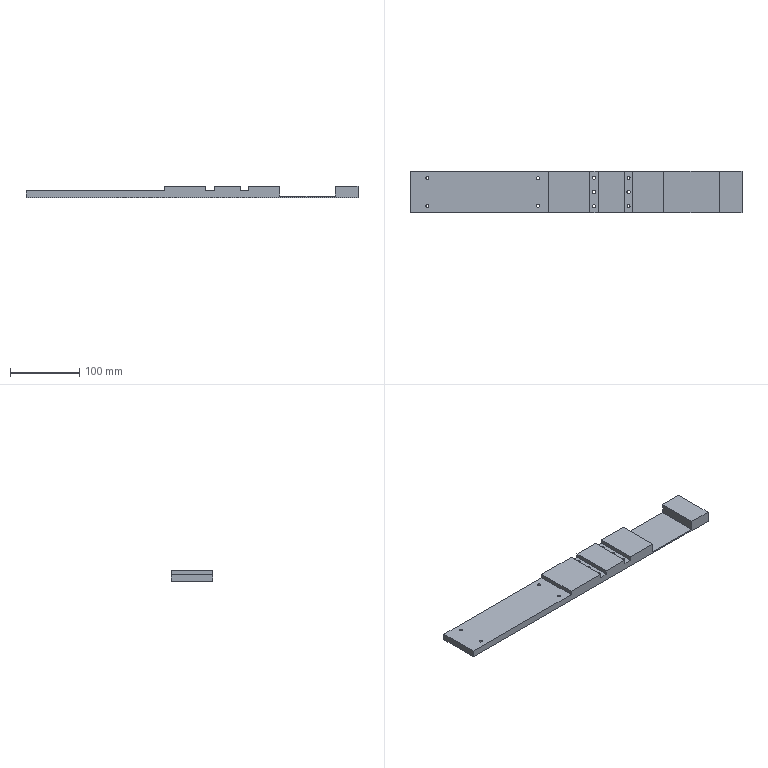Part | SolidWorks | features ICE 4, Extrusion 1 | 1 solid | 40 faces | box 480 x 60 x 16 mm | volume 311459 mm3 | cylinder 20 | plane 20 | commonest cylinder face diameters 4.2 x16 5 x4
STEP:
#1=CARTESIAN_POINT('',(-136.908,-22.163,0.));
#2=VERTEX_POINT('',#1);
#3=CARTESIAN_POINT('',(-132.708,-22.163,0.));
#4=VERTEX_POINT('',#3);
#5=CARTESIAN_POINT('',(-134.808,-22.163,0.));
#6=DIRECTION('',(0.,0.,1.));
#7=DIRECTION('',(1.,0.,0.));
#8=AXIS2_PLACEMENT_3D('',#5,#6,#7);
#9=CIRCLE('',#8,2.1);
#10=EDGE_CURVE('',#2,#4,#9,.T.);
#11=ORIENTED_EDGE('',*,*,#10,.F.);
#12=CARTESIAN_POINT('',(-136.908,-22.163,10.));
#13=VERTEX_POINT('',#12);
#14=CARTESIAN_POINT('',(-136.908,-22.163,0.));
#15=DIRECTION('',(0.,0.,1.));
#16=VECTOR('',#15,1000.);
#17=LINE('',#14,#16);
#18=EDGE_CURVE('',#2,#13,#17,.T.);
#19=ORIENTED_EDGE('',*,*,#18,.T.);
#20=CARTESIAN_POINT('',(-132.708,-22.163,10.));
#21=VERTEX_POINT('',#20);
#22=CARTESIAN_POINT('',(-134.808,-22.163,10.));
#23=DIRECTION('',(0.,0.,1.));
#24=DIRECTION('',(1.,0.,0.));
#25=AXIS2_PLACEMENT_3D('',#22,#23,#24);
#26=CIRCLE('',#25,2.1);
#27=EDGE_CURVE('',#13,#21,#26,.T.);
#28=ORIENTED_EDGE('',*,*,#27,.T.);
#29=CARTESIAN_POINT('',(-132.708,-22.163,0.));
#30=DIRECTION('',(0.,0.,1.));
#31=VECTOR('',#30,1000.);
#32=LINE('',#29,#31);
#33=EDGE_CURVE('',#4,#21,#32,.T.);
#34=ORIENTED_EDGE('',*,*,#33,.F.);
#35=EDGE_LOOP('',(#11,#19,#28,#34));
#36=FACE_OUTER_BOUND('',#35,.T.);
#37=CARTESIAN_POINT('',(-134.808,-22.163,0.));
#38=DIRECTION('',(0.,0.,1.));
#39=DIRECTION('',(1.,0.,0.));
#40=AXIS2_PLACEMENT_3D('',#37,#38,#39);
#41=CYLINDRICAL_SURFACE('',#40,2.1);
#42=ADVANCED_FACE('',(#36),#41,.F.);
#43=CARTESIAN_POINT('',(23.092,17.837,0.));
#44=VERTEX_POINT('',#43);
#45=CARTESIAN_POINT('',(27.292,17.837,0.));
#46=VERTEX_POINT('',#45);
#47=CARTESIAN_POINT('',(25.192,17.837,0.));
#48=DIRECTION('',(0.,0.,1.));
#49=DIRECTION('',(1.,0.,0.));
#50=AXIS2_PLACEMENT_3D('',#47,#48,#49);
#51=CIRCLE('',#50,2.1);
#52=EDGE_CURVE('',#44,#46,#51,.T.);
#53=ORIENTED_EDGE('',*,*,#52,.F.);
#54=CARTESIAN_POINT('',(23.092,17.837,10.));
#55=VERTEX_POINT('',#54);
#56=CARTESIAN_POINT('',(23.092,17.837,0.));
#57=DIRECTION('',(0.,0.,1.));
#58=VECTOR('',#57,1000.);
#59=LINE('',#56,#58);
#60=EDGE_CURVE('',#44,#55,#59,.T.);
#61=ORIENTED_EDGE('',*,*,#60,.T.);
#62=CARTESIAN_POINT('',(27.292,17.837,10.));
#63=VERTEX_POINT('',#62);
#64=CARTESIAN_POINT('',(25.192,17.837,10.));
#65=DIRECTION('',(0.,0.,1.));
#66=DIRECTION('',(1.,0.,0.));
#67=AXIS2_PLACEMENT_3D('',#64,#65,#66);
#68=CIRCLE('',#67,2.1);
#69=EDGE_CURVE('',#55,#63,#68,.T.);
#70=ORIENTED_EDGE('',*,*,#69,.T.);
#71=CARTESIAN_POINT('',(27.292,17.837,0.));
#72=DIRECTION('',(0.,0.,1.));
#73=VECTOR('',#72,1000.);
#74=LINE('',#71,#73);
#75=EDGE_CURVE('',#46,#63,#74,.T.);
#76=ORIENTED_EDGE('',*,*,#75,.F.);
#77=EDGE_LOOP('',(#53,#61,#70,#76));
#78=FACE_OUTER_BOUND('',#77,.T.);
#79=CARTESIAN_POINT('',(25.192,17.837,0.));
#80=DIRECTION('',(0.,0.,1.));
#81=DIRECTION('',(1.,0.,0.));
#82=AXIS2_PLACEMENT_3D('',#79,#80,#81);
#83=CYLINDRICAL_SURFACE('',#82,2.1);
#84=ADVANCED_FACE('',(#78),#83,.F.);
#85=CARTESIAN_POINT('',(23.092,-22.163,0.));
#86=VERTEX_POINT('',#85);
#87=CARTESIAN_POINT('',(27.292,-22.163,0.));
#88=VERTEX_POINT('',#87);
#89=CARTESIAN_POINT('',(25.192,-22.163,0.));
#90=DIRECTION('',(0.,0.,1.));
#91=DIRECTION('',(1.,0.,0.));
#92=AXIS2_PLACEMENT_3D('',#89,#90,#91);
#93=CIRCLE('',#92,2.1);
#94=EDGE_CURVE('',#86,#88,#93,.T.);
#95=ORIENTED_EDGE('',*,*,#94,.F.);
#96=CARTESIAN_POINT('',(23.092,-22.163,10.));
#97=VERTEX_POINT('',#96);
#98=CARTESIAN_POINT('',(23.092,-22.163,0.));
#99=DIRECTION('',(0.,0.,1.));
#100=VECTOR('',#99,1000.);
#101=LINE('',#98,#100);
#102=EDGE_CURVE('',#86,#97,#101,.T.);
#103=ORIENTED_EDGE('',*,*,#102,.T.);
#104=CARTESIAN_POINT('',(27.292,-22.163,10.));
#105=VERTEX_POINT('',#104);
#106=CARTESIAN_POINT('',(25.192,-22.163,10.));
#107=DIRECTION('',(0.,0.,1.));
#108=DIRECTION('',(1.,0.,0.));
#109=AXIS2_PLACEMENT_3D('',#106,#107,#108);
#110=CIRCLE('',#109,2.1);
#111=EDGE_CURVE('',#97,#105,#110,.T.);
#112=ORIENTED_EDGE('',*,*,#111,.T.);
#113=CARTESIAN_POINT('',(27.292,-22.163,0.));
#114=DIRECTION('',(0.,0.,1.));
#115=VECTOR('',#114,1000.);
#116=LINE('',#113,#115);
#117=EDGE_CURVE('',#88,#105,#116,.T.);
#118=ORIENTED_EDGE('',*,*,#117,.F.);
#119=EDGE_LOOP('',(#95,#103,#112,#118));
#120=FACE_OUTER_BOUND('',#119,.T.);
#121=CARTESIAN_POINT('',(25.192,-22.163,0.));
#122=DIRECTION('',(0.,0.,1.));
#123=DIRECTION('',(1.,0.,0.));
#124=AXIS2_PLACEMENT_3D('',#121,#122,#123);
#125=CYLINDRICAL_SURFACE('',#124,2.1);
#126=ADVANCED_FACE('',(#120),#125,.F.);
#127=CARTESIAN_POINT('',(-136.908,17.837,0.));
#128=VERTEX_POINT('',#127);
#129=CARTESIAN_POINT('',(-132.708,17.837,0.));
#130=VERTEX_POINT('',#129);
#131=CARTESIAN_POINT('',(-134.808,17.837,0.));
#132=DIRECTION('',(0.,0.,1.));
#133=DIRECTION('',(1.,0.,0.));
#134=AXIS2_PLACEMENT_3D('',#131,#132,#133);
#135=CIRCLE('',#134,2.1);
#136=EDGE_CURVE('',#128,#130,#135,.T.);
#137=ORIENTED_EDGE('',*,*,#136,.F.);
#138=CARTESIAN_POINT('',(-136.908,17.837,10.));
#139=VERTEX_POINT('',#138);
#140=CARTESIAN_POINT('',(-136.908,17.837,0.));
#141=DIRECTION('',(0.,0.,1.));
#142=VECTOR('',#141,1000.);
#143=LINE('',#140,#142);
#144=EDGE_CURVE('',#128,#139,#143,.T.);
#145=ORIENTED_EDGE('',*,*,#144,.T.);
#146=CARTESIAN_POINT('',(-132.708,17.837,10.));
#147=VERTEX_POINT('',#146);
#148=CARTESIAN_POINT('',(-134.808,17.837,10.));
#149=DIRECTION('',(0.,0.,1.));
#150=DIRECTION('',(1.,0.,0.));
#151=AXIS2_PLACEMENT_3D('',#148,#149,#150);
#152=CIRCLE('',#151,2.1);
#153=EDGE_CURVE('',#139,#147,#152,.T.);
#154=ORIENTED_EDGE('',*,*,#153,.T.);
#155=CARTESIAN_POINT('',(-132.708,17.837,0.));
#156=DIRECTION('',(0.,0.,1.));
#157=VECTOR('',#156,1000.);
#158=LINE('',#155,#157);
#159=EDGE_CURVE('',#130,#147,#158,.T.);
#160=ORIENTED_EDGE('',*,*,#159,.F.);
#161=EDGE_LOOP('',(#137,#145,#154,#160));
#162=FACE_OUTER_BOUND('',#161,.T.);
#163=CARTESIAN_POINT('',(-134.808,17.837,0.));
#164=DIRECTION('',(0.,0.,1.));
#165=DIRECTION('',(1.,0.,0.));
#166=AXIS2_PLACEMENT_3D('',#163,#164,#165);
#167=CYLINDRICAL_SURFACE('',#166,2.1);
#168=ADVANCED_FACE('',(#162),#167,.F.);
#169=CARTESIAN_POINT('',(154.092,18.337,0.));
#170=VERTEX_POINT('',#169);
#171=CARTESIAN_POINT('',(158.292,18.337,0.));
#172=VERTEX_POINT('',#171);
#173=CARTESIAN_POINT('',(156.192,18.337,0.));
#174=DIRECTION('',(0.,0.,1.));
#175=DIRECTION('',(1.,0.,0.));
#176=AXIS2_PLACEMENT_3D('',#173,#174,#175);
#177=CIRCLE('',#176,2.1);
#178=EDGE_CURVE('',#170,#172,#177,.T.);
#179=ORIENTED_EDGE('',*,*,#178,.F.);
#180=CARTESIAN_POINT('',(154.092,18.337,10.));
#181=VERTEX_POINT('',#180);
#182=CARTESIAN_POINT('',(154.092,18.337,0.));
#183=DIRECTION('',(0.,0.,1.));
#184=VECTOR('',#183,1000.);
#185=LINE('',#182,#184);
#186=EDGE_CURVE('',#170,#181,#185,.T.);
#187=ORIENTED_EDGE('',*,*,#186,.T.);
#188=CARTESIAN_POINT('',(158.292,18.337,10.));
#189=VERTEX_POINT('',#188);
#190=CARTESIAN_POINT('',(156.192,18.337,10.));
#191=DIRECTION('',(0.,0.,1.));
#192=DIRECTION('',(1.,0.,0.));
#193=AXIS2_PLACEMENT_3D('',#190,#191,#192);
#194=CIRCLE('',#193,2.1);
#195=EDGE_CURVE('',#181,#189,#194,.T.);
#196=ORIENTED_EDGE('',*,*,#195,.T.);
#197=CARTESIAN_POINT('',(158.292,18.337,0.));
#198=DIRECTION('',(0.,0.,1.));
#199=VECTOR('',#198,1000.);
#200=LINE('',#197,#199);
#201=EDGE_CURVE('',#172,#189,#200,.T.);
#202=ORIENTED_EDGE('',*,*,#201,.F.);
#203=EDGE_LOOP('',(#179,#187,#196,#202));
#204=FACE_OUTER_BOUND('',#203,.T.);
#205=CARTESIAN_POINT('',(156.192,18.337,0.));
#206=DIRECTION('',(0.,0.,1.));
#207=DIRECTION('',(1.,0.,0.));
#208=AXIS2_PLACEMENT_3D('',#205,#206,#207);
#209=CYLINDRICAL_SURFACE('',#208,2.1);
#210=ADVANCED_FACE('',(#204),#209,.F.);
#211=CARTESIAN_POINT('',(154.092,-22.663,0.));
#212=VERTEX_POINT('',#211);
#213=CARTESIAN_POINT('',(158.292,-22.663,0.));
#214=VERTEX_POINT('',#213);
#215=CARTESIAN_POINT('',(156.192,-22.663,0.));
#216=DIRECTION('',(0.,0.,1.));
#217=DIRECTION('',(1.,0.,0.));
#218=AXIS2_PLACEMENT_3D('',#215,#216,#217);
#219=CIRCLE('',#218,2.1);
#220=EDGE_CURVE('',#212,#214,#219,.T.);
#221=ORIENTED_EDGE('',*,*,#220,.F.);
#222=CARTESIAN_POINT('',(154.092,-22.663,10.));
#223=VERTEX_POINT('',#222);
#224=CARTESIAN_POINT('',(154.092,-22.663,0.));
#225=DIRECTION('',(0.,0.,1.));
#226=VECTOR('',#225,1000.);
#227=LINE('',#224,#226);
#228=EDGE_CURVE('',#212,#223,#227,.T.);
#229=ORIENTED_EDGE('',*,*,#228,.T.);
#230=CARTESIAN_POINT('',(158.292,-22.663,10.));
#231=VERTEX_POINT('',#230);
#232=CARTESIAN_POINT('',(156.192,-22.663,10.));
#233=DIRECTION('',(0.,0.,1.));
#234=DIRECTION('',(1.,0.,0.));
#235=AXIS2_PLACEMENT_3D('',#232,#233,#234);
#236=CIRCLE('',#235,2.1);
#237=EDGE_CURVE('',#223,#231,#236,.T.);
#238=ORIENTED_EDGE('',*,*,#237,.T.);
#239=CARTESIAN_POINT('',(158.292,-22.663,0.));
#240=DIRECTION('',(0.,0.,1.));
#241=VECTOR('',#240,1000.);
#242=LINE('',#239,#241);
#243=EDGE_CURVE('',#214,#231,#242,.T.);
#244=ORIENTED_EDGE('',*,*,#243,.F.);
#245=EDGE_LOOP('',(#221,#229,#238,#244));
#246=FACE_OUTER_BOUND('',#245,.T.);
#247=CARTESIAN_POINT('',(156.192,-22.663,0.));
#248=DIRECTION('',(0.,0.,1.));
#249=DIRECTION('',(1.,0.,0.));
#250=AXIS2_PLACEMENT_3D('',#247,#248,#249);
#251=CYLINDRICAL_SURFACE('',#250,2.1);
#252=ADVANCED_FACE('',(#246),#251,.F.);
#253=CARTESIAN_POINT('',(153.692,-2.163,0.));
#254=VERTEX_POINT('',#253);
#255=CARTESIAN_POINT('',(158.692,-2.163,0.));
#256=VERTEX_POINT('',#255);
#257=CARTESIAN_POINT('',(156.192,-2.163,0.));
#258=DIRECTION('',(0.,0.,1.));
#259=DIRECTION('',(1.,0.,0.));
#260=AXIS2_PLACEMENT_3D('',#257,#258,#259);
#261=CIRCLE('',#260,2.5);
#262=EDGE_CURVE('',#254,#256,#261,.T.);
#263=ORIENTED_EDGE('',*,*,#262,.F.);
#264=CARTESIAN_POINT('',(153.692,-2.163,10.));
#265=VERTEX_POINT('',#264);
#266=CARTESIAN_POINT('',(153.692,-2.163,0.));
#267=DIRECTION('',(0.,0.,1.));
#268=VECTOR('',#267,1000.);
#269=LINE('',#266,#268);
#270=EDGE_CURVE('',#254,#265,#269,.T.);
#271=ORIENTED_EDGE('',*,*,#270,.T.);
#272=CARTESIAN_POINT('',(158.692,-2.163,10.));
#273=VERTEX_POINT('',#272);
#274=CARTESIAN_POINT('',(156.192,-2.163,10.));
#275=DIRECTION('',(0.,0.,1.));
#276=DIRECTION('',(1.,0.,0.));
#277=AXIS2_PLACEMENT_3D('',#274,#275,#276);
#278=CIRCLE('',#277,2.5);
#279=EDGE_CURVE('',#265,#273,#278,.T.);
#280=ORIENTED_EDGE('',*,*,#279,.T.);
#281=CARTESIAN_POINT('',(158.692,-2.163,0.));
#282=DIRECTION('',(0.,0.,1.));
#283=VECTOR('',#282,1000.);
#284=LINE('',#281,#283);
#285=EDGE_CURVE('',#256,#273,#284,.T.);
#286=ORIENTED_EDGE('',*,*,#285,.F.);
#287=EDGE_LOOP('',(#263,#271,#280,#286));
#288=FACE_OUTER_BOUND('',#287,.T.);
#289=CARTESIAN_POINT('',(156.192,-2.163,0.));
#290=DIRECTION('',(0.,0.,1.));
#291=DIRECTION('',(1.,0.,0.));
#292=AXIS2_PLACEMENT_3D('',#289,#290,#291);
#293=CYLINDRICAL_SURFACE('',#292,2.5);
#294=ADVANCED_FACE('',(#288),#293,.F.);
#295=CARTESIAN_POINT('',(104.092,-22.663,0.));
#296=VERTEX_POINT('',#295);
#297=CARTESIAN_POINT('',(108.292,-22.663,0.));
#298=VERTEX_POINT('',#297);
#299=CARTESIAN_POINT('',(106.192,-22.663,0.));
#300=DIRECTION('',(0.,0.,1.));
#301=DIRECTION('',(1.,0.,0.));
#302=AXIS2_PLACEMENT_3D('',#299,#300,#301);
#303=CIRCLE('',#302,2.1);
#304=EDGE_CURVE('',#296,#298,#303,.T.);
#305=ORIENTED_EDGE('',*,*,#304,.F.);
#306=CARTESIAN_POINT('',(104.092,-22.663,10.));
#307=VERTEX_POINT('',#306);
#308=CARTESIAN_POINT('',(104.092,-22.663,0.));
#309=DIRECTION('',(0.,0.,1.));
#310=VECTOR('',#309,1000.);
#311=LINE('',#308,#310);
#312=EDGE_CURVE('',#296,#307,#311,.T.);
#313=ORIENTED_EDGE('',*,*,#312,.T.);
#314=CARTESIAN_POINT('',(108.292,-22.663,10.));
#315=VERTEX_POINT('',#314);
#316=CARTESIAN_POINT('',(106.192,-22.663,10.));
#317=DIRECTION('',(0.,0.,1.));
#318=DIRECTION('',(1.,0.,0.));
#319=AXIS2_PLACEMENT_3D('',#316,#317,#318);
#320=CIRCLE('',#319,2.1);
#321=EDGE_CURVE('',#307,#315,#320,.T.);
#322=ORIENTED_EDGE('',*,*,#321,.T.);
#323=CARTESIAN_POINT('',(108.292,-22.663,0.));
#324=DIRECTION('',(0.,0.,1.));
#325=VECTOR('',#324,1000.);
#326=LINE('',#323,#325);
#327=EDGE_CURVE('',#298,#315,#326,.T.);
#328=ORIENTED_EDGE('',*,*,#327,.F.);
#329=EDGE_LOOP('',(#305,#313,#322,#328));
#330=FACE_OUTER_BOUND('',#329,.T.);
#331=CARTESIAN_POINT('',(106.192,-22.663,0.));
#332=DIRECTION('',(0.,0.,1.));
#333=DIRECTION('',(1.,0.,0.));
#334=AXIS2_PLACEMENT_3D('',#331,#332,#333);
#335=CYLINDRICAL_SURFACE('',#334,2.1);
#336=ADVANCED_FACE('',(#330),#335,.F.);
#337=CARTESIAN_POINT('',(103.692,-2.163,0.));
#338=VERTEX_POINT('',#337);
#339=CARTESIAN_POINT('',(108.692,-2.163,0.));
#340=VERTEX_POINT('',#339);
#341=CARTESIAN_POINT('',(106.192,-2.163,0.));
#342=DIRECTION('',(0.,0.,1.));
#343=DIRECTION('',(1.,0.,0.));
#344=AXIS2_PLACEMENT_3D('',#341,#342,#343);
#345=CIRCLE('',#344,2.5);
#346=EDGE_CURVE('',#338,#340,#345,.T.);
#347=ORIENTED_EDGE('',*,*,#346,.F.);
#348=CARTESIAN_POINT('',(103.692,-2.163,10.));
#349=VERTEX_POINT('',#348);
#350=CARTESIAN_POINT('',(103.692,-2.163,0.));
#351=DIRECTION('',(0.,0.,1.));
#352=VECTOR('',#351,1000.);
#353=LINE('',#350,#352);
#354=EDGE_CURVE('',#338,#349,#353,.T.);
#355=ORIENTED_EDGE('',*,*,#354,.T.);
#356=CARTESIAN_POINT('',(108.692,-2.163,10.));
#357=VERTEX_POINT('',#356);
#358=CARTESIAN_POINT('',(106.192,-2.163,10.));
#359=DIRECTION('',(0.,0.,1.));
#360=DIRECTION('',(1.,0.,0.));
#361=AXIS2_PLACEMENT_3D('',#358,#359,#360);
#362=CIRCLE('',#361,2.5);
#363=EDGE_CURVE('',#349,#357,#362,.T.);
#364=ORIENTED_EDGE('',*,*,#363,.T.);
#365=CARTESIAN_POINT('',(108.692,-2.163,0.));
#366=DIRECTION('',(0.,0.,1.));
#367=VECTOR('',#366,1000.);
#368=LINE('',#365,#367);
#369=EDGE_CURVE('',#340,#357,#368,.T.);
#370=ORIENTED_EDGE('',*,*,#369,.F.);
#371=EDGE_LOOP('',(#347,#355,#364,#370));
#372=FACE_OUTER_BOUND('',#371,.T.);
#373=CARTESIAN_POINT('',(106.192,-2.163,0.));
#374=DIRECTION('',(0.,0.,1.));
#375=DIRECTION('',(1.,0.,0.));
#376=AXIS2_PLACEMENT_3D('',#373,#374,#375);
#377=CYLINDRICAL_SURFACE('',#376,2.5);
#378=ADVANCED_FACE('',(#372),#377,.F.);
#379=CARTESIAN_POINT('',(104.092,18.337,0.));
#380=VERTEX_POINT('',#379);
#381=CARTESIAN_POINT('',(108.292,18.337,0.));
#382=VERTEX_POINT('',#381);
#383=CARTESIAN_POINT('',(106.192,18.337,0.));
#384=DIRECTION('',(0.,0.,1.));
#385=DIRECTION('',(1.,0.,0.));
#386=AXIS2_PLACEMENT_3D('',#383,#384,#385);
#387=CIRCLE('',#386,2.1);
#388=EDGE_CURVE('',#380,#382,#387,.T.);
#389=ORIENTED_EDGE('',*,*,#388,.F.);
#390=CARTESIAN_POINT('',(104.092,18.337,10.));
#391=VERTEX_POINT('',#390);
#392=CARTESIAN_POINT('',(104.092,18.337,0.));
#393=DIRECTION('',(0.,0.,1.));
#394=VECTOR('',#393,1000.);
#395=LINE('',#392,#394);
#396=EDGE_CURVE('',#380,#391,#395,.T.);
#397=ORIENTED_EDGE('',*,*,#396,.T.);
#398=CARTESIAN_POINT('',(108.292,18.337,10.));
#399=VERTEX_POINT('',#398);
#400=CARTESIAN_POINT('',(106.192,18.337,10.));
#401=DIRECTION('',(0.,0.,1.));
#402=DIRECTION('',(1.,0.,0.));
#403=AXIS2_PLACEMENT_3D('',#400,#401,#402);
#404=CIRCLE('',#403,2.1);
#405=EDGE_CURVE('',#391,#399,#404,.T.);
#406=ORIENTED_EDGE('',*,*,#405,.T.);
#407=CARTESIAN_POINT('',(108.292,18.337,0.));
#408=DIRECTION('',(0.,0.,1.));
#409=VECTOR('',#408,1000.);
#410=LINE('',#407,#409);
#411=EDGE_CURVE('',#382,#399,#410,.T.);
#412=ORIENTED_EDGE('',*,*,#411,.F.);
#413=EDGE_LOOP('',(#389,#397,#406,#412));
#414=FACE_OUTER_BOUND('',#413,.T.);
#415=CARTESIAN_POINT('',(106.192,18.337,0.));
#416=DIRECTION('',(0.,0.,1.));
#417=DIRECTION('',(1.,0.,0.));
#418=AXIS2_PLACEMENT_3D('',#415,#416,#417);
#419=CYLINDRICAL_SURFACE('',#418,2.1);
#420=ADVANCED_FACE('',(#414),#419,.F.);
#421=CARTESIAN_POINT('',(287.192,-32.163,16.));
#422=VERTEX_POINT('',#421);
#423=CARTESIAN_POINT('',(287.192,27.837,16.));
#424=VERTEX_POINT('',#423);
#425=CARTESIAN_POINT('',(287.192,-32.163,16.));
#426=DIRECTION('',(0.,1.,0.));
#427=VECTOR('',#426,1000.);
#428=LINE('',#425,#427);
#429=EDGE_CURVE('',#422,#424,#428,.T.);
#430=ORIENTED_EDGE('',*,*,#429,.F.);
#431=CARTESIAN_POINT('',(320.192,-32.163,16.));
#432=VERTEX_POINT('',#431);
#433=CARTESIAN_POINT('',(320.192,-32.163,16.));
#434=DIRECTION('',(1.,0.,0.));
#435=VECTOR('',#434,1000.);
#436=LINE('',#433,#435);
#437=EDGE_CURVE('',#422,#432,#436,.T.);
#438=ORIENTED_EDGE('',*,*,#437,.T.);
#439=CARTESIAN_POINT('',(320.192,27.837,16.));
#440=VERTEX_POINT('',#439);
#441=CARTESIAN_POINT('',(320.192,-32.163,16.));
#442=DIRECTION('',(0.,1.,0.));
#443=VECTOR('',#442,1000.);
#444=LINE('',#441,#443);
#445=EDGE_CURVE('',#432,#440,#444,.T.);
#446=ORIENTED_EDGE('',*,*,#445,.T.);
#447=CARTESIAN_POINT('',(320.192,27.837,16.));
#448=DIRECTION('',(-1.,0.,0.));
#449=VECTOR('',#448,1000.);
#450=LINE('',#447,#449);
#451=EDGE_CURVE('',#440,#424,#450,.T.);
#452=ORIENTED_EDGE('',*,*,#451,.T.);
#453=EDGE_LOOP('',(#430,#438,#446,#452));
#454=FACE_OUTER_BOUND('',#453,.T.);
#455=CARTESIAN_POINT('',(0.,0.,16.));
#456=DIRECTION('',(0.,0.,1.));
#457=DIRECTION('',(1.,0.,0.));
#458=AXIS2_PLACEMENT_3D('',#455,#456,#457);
#459=PLANE('',#458);
#460=ADVANCED_FACE('',(#454),#459,.T.);
#461=CARTESIAN_POINT('',(100.192,27.837,16.));
#462=VERTEX_POINT('',#461);
#463=CARTESIAN_POINT('',(100.192,-32.163,16.));
#464=VERTEX_POINT('',#463);
#465=CARTESIAN_POINT('',(100.192,-32.163,16.));
#466=DIRECTION('',(0.,-1.,0.));
#467=VECTOR('',#466,1000.);
#468=LINE('',#465,#467);
#469=EDGE_CURVE('',#462,#464,#468,.T.);
#470=ORIENTED_EDGE('',*,*,#469,.F.);
#471=CARTESIAN_POINT('',(40.192,27.837,16.));
#472=VERTEX_POINT('',#471);
#473=CARTESIAN_POINT('',(320.192,27.837,16.));
#474=DIRECTION('',(-1.,0.,0.));
#475=VECTOR('',#474,1000.);
#476=LINE('',#473,#475);
#477=EDGE_CURVE('',#462,#472,#476,.T.);
#478=ORIENTED_EDGE('',*,*,#477,.T.);
#479=CARTESIAN_POINT('',(40.192,-32.163,16.));
#480=VERTEX_POINT('',#479);
#481=CARTESIAN_POINT('',(40.192,27.837,16.));
#482=DIRECTION('',(0.,1.,0.));
#483=VECTOR('',#482,1000.);
#484=LINE('',#481,#483);
#485=EDGE_CURVE('',#480,#472,#484,.T.);
#486=ORIENTED_EDGE('',*,*,#485,.F.);
#487=CARTESIAN_POINT('',(320.192,-32.163,16.));
#488=DIRECTION('',(1.,0.,0.));
#489=VECTOR('',#488,1000.);
#490=LINE('',#487,#489);
#491=EDGE_CURVE('',#480,#464,#490,.T.);
#492=ORIENTED_EDGE('',*,*,#491,.T.);
#493=EDGE_LOOP('',(#470,#478,#486,#492));
#494=FACE_OUTER_BOUND('',#493,.T.);
#495=CARTESIAN_POINT('',(0.,0.,16.));
#496=DIRECTION('',(0.,0.,1.));
#497=DIRECTION('',(1.,0.,0.));
#498=AXIS2_PLACEMENT_3D('',#495,#496,#497);
#499=PLANE('',#498);
#500=ADVANCED_FACE('',(#494),#499,.T.);
#501=CARTESIAN_POINT('',(112.192,-32.163,16.));
#502=VERTEX_POINT('',#501);
#503=CARTESIAN_POINT('',(112.192,27.837,16.));
#504=VERTEX_POINT('',#503);
#505=CARTESIAN_POINT('',(112.192,27.837,16.));
#506=DIRECTION('',(0.,1.,0.));
#507=VECTOR('',#506,1000.);
#508=LINE('',#505,#507);
#509=EDGE_CURVE('',#502,#504,#508,.T.);
#510=ORIENTED_EDGE('',*,*,#509,.F.);
#511=CARTESIAN_POINT('',(150.192,-32.163,16.));
#512=VERTEX_POINT('',#511);
#513=CARTESIAN_POINT('',(320.192,-32.163,16.));
#514=DIRECTION('',(1.,0.,0.));
#515=VECTOR('',#514,1000.);
#516=LINE('',#513,#515);
#517=EDGE_CURVE('',#502,#512,#516,.T.);
#518=ORIENTED_EDGE('',*,*,#517,.T.);
#519=CARTESIAN_POINT('',(150.192,27.837,16.));
#520=VERTEX_POINT('',#519);
#521=CARTESIAN_POINT('',(150.192,27.837,16.));
#522=DIRECTION('',(0.,-1.,0.));
#523=VECTOR('',#522,1000.);
#524=LINE('',#521,#523);
#525=EDGE_CURVE('',#520,#512,#524,.T.);
#526=ORIENTED_EDGE('',*,*,#525,.F.);
#527=CARTESIAN_POINT('',(320.192,27.837,16.));
#528=DIRECTION('',(-1.,0.,0.));
#529=VECTOR('',#528,1000.);
#530=LINE('',#527,#529);
#531=EDGE_CURVE('',#520,#504,#530,.T.);
#532=ORIENTED_EDGE('',*,*,#531,.T.);
#533=EDGE_LOOP('',(#510,#518,#526,#532));
#534=FACE_OUTER_BOUND('',#533,.T.);
#535=CARTESIAN_POINT('',(0.,0.,16.));
#536=DIRECTION('',(0.,0.,1.));
#537=DIRECTION('',(1.,0.,0.));
#538=AXIS2_PLACEMENT_3D('',#535,#536,#537);
#539=PLANE('',#538);
#540=ADVANCED_FACE('',(#534),#539,.T.);
#541=CARTESIAN_POINT('',(-159.808,27.837,10.));
#542=VERTEX_POINT('',#541);
#543=CARTESIAN_POINT('',(-159.808,-32.163,10.));
#544=VERTEX_POINT('',#543);
#545=CARTESIAN_POINT('',(-159.808,27.837,10.));
#546=DIRECTION('',(0.,-1.,0.));
#547=VECTOR('',#546,1000.);
#548=LINE('',#545,#547);
#549=EDGE_CURVE('',#542,#544,#548,.T.);
#550=ORIENTED_EDGE('',*,*,#549,.F.);
#551=CARTESIAN_POINT('',(-159.808,27.837,0.));
#552=VERTEX_POINT('',#551);
#553=CARTESIAN_POINT('',(-159.808,27.837,16.));
#554=DIRECTION('',(0.,0.,-1.));
#555=VECTOR('',#554,1000.);
#556=LINE('',#553,#555);
#557=EDGE_CURVE('',#542,#552,#556,.T.);
#558=ORIENTED_EDGE('',*,*,#557,.T.);
#559=CARTESIAN_POINT('',(-159.808,-32.163,0.));
#560=VERTEX_POINT('',#559);
#561=CARTESIAN_POINT('',(-159.808,-32.163,0.));
#562=DIRECTION('',(0.,-1.,0.));
#563=VECTOR('',#562,1000.);
#564=LINE('',#561,#563);
#565=EDGE_CURVE('',#552,#560,#564,.T.);
#566=ORIENTED_EDGE('',*,*,#565,.T.);
#567=CARTESIAN_POINT('',(-159.808,-32.163,16.));
#568=DIRECTION('',(0.,0.,-1.));
#569=VECTOR('',#568,1000.);
#570=LINE('',#567,#569);
#571=EDGE_CURVE('',#544,#560,#570,.T.);
#572=ORIENTED_EDGE('',*,*,#571,.F.);
#573=EDGE_LOOP('',(#550,#558,#566,#572));
#574=FACE_OUTER_BOUND('',#573,.T.);
#575=CARTESIAN_POINT('',(-159.808,-32.163,16.));
#576=DIRECTION('',(1.,0.,0.));
#577=DIRECTION('',(0.,0.,-1.));
#578=AXIS2_PLACEMENT_3D('',#575,#576,#577);
#579=PLANE('',#578);
#580=ADVANCED_FACE('',(#574),#579,.F.);
#581=CARTESIAN_POINT('',(320.192,-32.163,0.));
#582=VERTEX_POINT('',#581);
#583=CARTESIAN_POINT('',(320.192,27.837,0.));
#584=VERTEX_POINT('',#583);
#585=CARTESIAN_POINT('',(320.192,-32.163,0.));
#586=DIRECTION('',(0.,1.,0.));
#587=VECTOR('',#586,1000.);
#588=LINE('',#585,#587);
#589=EDGE_CURVE('',#582,#584,#588,.T.);
#590=ORIENTED_EDGE('',*,*,#589,.T.);
#591=CARTESIAN_POINT('',(320.192,27.837,16.));
#592=DIRECTION('',(0.,0.,-1.));
#593=VECTOR('',#592,1000.);
#594=LINE('',#591,#593);
#595=EDGE_CURVE('',#440,#584,#594,.T.);
#596=ORIENTED_EDGE('',*,*,#595,.F.);
#597=ORIENTED_EDGE('',*,*,#445,.F.);
#598=CARTESIAN_POINT('',(320.192,-32.163,16.));
#599=DIRECTION('',(0.,0.,-1.));
#600=VECTOR('',#599,1000.);
#601=LINE('',#598,#600);
#602=EDGE_CURVE('',#432,#582,#601,.T.);
#603=ORIENTED_EDGE('',*,*,#602,.T.);
#604=EDGE_LOOP('',(#590,#596,#597,#603));
#605=FACE_OUTER_BOUND('',#604,.T.);
#606=CARTESIAN_POINT('',(320.192,-32.163,16.));
#607=DIRECTION('',(-1.,0.,0.));
#608=DIRECTION('',(0.,0.,1.));
#609=AXIS2_PLACEMENT_3D('',#606,#607,#608);
#610=PLANE('',#609);
#611=ADVANCED_FACE('',(#605),#610,.F.);
#612=CARTESIAN_POINT('',(287.192,27.837,2.));
#613=VERTEX_POINT('',#612);
#614=CARTESIAN_POINT('',(207.192,27.837,2.));
#615=VERTEX_POINT('',#614);
#616=CARTESIAN_POINT('',(287.192,27.837,2.));
#617=DIRECTION('',(-1.,0.,0.));
#618=VECTOR('',#617,1000.);
#619=LINE('',#616,#618);
#620=EDGE_CURVE('',#613,#615,#619,.T.);
#621=ORIENTED_EDGE('',*,*,#620,.F.);
#622=CARTESIAN_POINT('',(287.192,27.837,2.));
#623=DIRECTION('',(0.,0.,1.));
#624=VECTOR('',#623,1000.);
#625=LINE('',#622,#624);
#626=EDGE_CURVE('',#613,#424,#625,.T.);
#627=ORIENTED_EDGE('',*,*,#626,.T.);
#628=ORIENTED_EDGE('',*,*,#451,.F.);
#629=ORIENTED_EDGE('',*,*,#595,.T.);
#630=CARTESIAN_POINT('',(320.192,27.837,0.));
#631=DIRECTION('',(-1.,0.,0.));
#632=VECTOR('',#631,1000.);
#633=LINE('',#630,#632);
#634=EDGE_CURVE('',#584,#552,#633,.T.);
#635=ORIENTED_EDGE('',*,*,#634,.T.);
#636=ORIENTED_EDGE('',*,*,#557,.F.);
#637=CARTESIAN_POINT('',(40.192,27.837,10.));
#638=VERTEX_POINT('',#637);
#639=CARTESIAN_POINT('',(-159.808,27.837,10.));
#640=DIRECTION('',(-1.,0.,0.));
#641=VECTOR('',#640,1000.);
#642=LINE('',#639,#641);
#643=EDGE_CURVE('',#638,#542,#642,.T.);
#644=ORIENTED_EDGE('',*,*,#643,.F.);
#645=CARTESIAN_POINT('',(40.192,27.837,10.));
#646=DIRECTION('',(0.,0.,1.));
#647=VECTOR('',#646,1000.);
#648=LINE('',#645,#647);
#649=EDGE_CURVE('',#638,#472,#648,.T.);
#650=ORIENTED_EDGE('',*,*,#649,.T.);
#651=ORIENTED_EDGE('',*,*,#477,.F.);
#652=CARTESIAN_POINT('',(100.192,27.837,10.));
#653=VERTEX_POINT('',#652);
#654=CARTESIAN_POINT('',(100.192,27.837,10.));
#655=DIRECTION('',(0.,0.,1.));
#656=VECTOR('',#655,1000.);
#657=LINE('',#654,#656);
#658=EDGE_CURVE('',#653,#462,#657,.T.);
#659=ORIENTED_EDGE('',*,*,#658,.F.);
#660=CARTESIAN_POINT('',(112.192,27.837,10.));
#661=VERTEX_POINT('',#660);
#662=CARTESIAN_POINT('',(100.192,27.837,10.));
#663=DIRECTION('',(-1.,0.,0.));
#664=VECTOR('',#663,1000.);
#665=LINE('',#662,#664);
#666=EDGE_CURVE('',#661,#653,#665,.T.);
#667=ORIENTED_EDGE('',*,*,#666,.F.);
#668=CARTESIAN_POINT('',(112.192,27.837,10.));
#669=DIRECTION('',(0.,0.,1.));
#670=VECTOR('',#669,1000.);
#671=LINE('',#668,#670);
#672=EDGE_CURVE('',#661,#504,#671,.T.);
#673=ORIENTED_EDGE('',*,*,#672,.T.);
#674=ORIENTED_EDGE('',*,*,#531,.F.);
#675=CARTESIAN_POINT('',(150.192,27.837,10.));
#676=VERTEX_POINT('',#675);
#677=CARTESIAN_POINT('',(150.192,27.837,10.));
#678=DIRECTION('',(0.,0.,1.));
#679=VECTOR('',#678,1000.);
#680=LINE('',#677,#679);
#681=EDGE_CURVE('',#676,#520,#680,.T.);
#682=ORIENTED_EDGE('',*,*,#681,.F.);
#683=CARTESIAN_POINT('',(162.192,27.837,10.));
#684=VERTEX_POINT('',#683);
#685=CARTESIAN_POINT('',(150.192,27.837,10.));
#686=DIRECTION('',(-1.,0.,0.));
#687=VECTOR('',#686,1000.);
#688=LINE('',#685,#687);
#689=EDGE_CURVE('',#684,#676,#688,.T.);
#690=ORIENTED_EDGE('',*,*,#689,.F.);
#691=CARTESIAN_POINT('',(162.192,27.837,16.));
#692=VERTEX_POINT('',#691);
#693=CARTESIAN_POINT('',(162.192,27.837,10.));
#694=DIRECTION('',(0.,0.,1.));
#695=VECTOR('',#694,1000.);
#696=LINE('',#693,#695);
#697=EDGE_CURVE('',#684,#692,#696,.T.);
#698=ORIENTED_EDGE('',*,*,#697,.T.);
#699=CARTESIAN_POINT('',(207.192,27.837,16.));
#700=VERTEX_POINT('',#699);
#701=CARTESIAN_POINT('',(320.192,27.837,16.));
#702=DIRECTION('',(-1.,0.,0.));
#703=VECTOR('',#702,1000.);
#704=LINE('',#701,#703);
#705=EDGE_CURVE('',#700,#692,#704,.T.);
#706=ORIENTED_EDGE('',*,*,#705,.F.);
#707=CARTESIAN_POINT('',(207.192,27.837,2.));
#708=DIRECTION('',(0.,0.,1.));
#709=VECTOR('',#708,1000.);
#710=LINE('',#707,#709);
#711=EDGE_CURVE('',#615,#700,#710,.T.);
#712=ORIENTED_EDGE('',*,*,#711,.F.);
#713=EDGE_LOOP('',(#621,#627,#628,#629,#635,#636,#644,#650,#651,#659,#667,#673,#674,#682,#690,#698,#706,#712));
#714=FACE_OUTER_BOUND('',#713,.T.);
#715=CARTESIAN_POINT('',(320.192,27.837,16.));
#716=DIRECTION('',(0.,-1.,0.));
#717=DIRECTION('',(1.,0.,0.));
#718=AXIS2_PLACEMENT_3D('',#715,#716,#717);
#719=PLANE('',#718);
#720=ADVANCED_FACE('',(#714),#719,.F.);
#721=ORIENTED_EDGE('',*,*,#437,.F.);
#722=CARTESIAN_POINT('',(287.192,-32.163,2.));
#723=VERTEX_POINT('',#722);
#724=CARTESIAN_POINT('',(287.192,-32.163,2.));
#725=DIRECTION('',(0.,0.,1.));
#726=VECTOR('',#725,1000.);
#727=LINE('',#724,#726);
#728=EDGE_CURVE('',#723,#422,#727,.T.);
#729=ORIENTED_EDGE('',*,*,#728,.F.);
#730=CARTESIAN_POINT('',(207.192,-32.163,2.));
#731=VERTEX_POINT('',#730);
#732=CARTESIAN_POINT('',(207.192,-32.163,2.));
#733=DIRECTION('',(1.,0.,0.));
#734=VECTOR('',#733,1000.);
#735=LINE('',#732,#734);
#736=EDGE_CURVE('',#731,#723,#735,.T.);
#737=ORIENTED_EDGE('',*,*,#736,.F.);
#738=CARTESIAN_POINT('',(207.192,-32.163,16.));
#739=VERTEX_POINT('',#738);
#740=CARTESIAN_POINT('',(207.192,-32.163,2.));
#741=DIRECTION('',(0.,0.,1.));
#742=VECTOR('',#741,1000.);
#743=LINE('',#740,#742);
#744=EDGE_CURVE('',#731,#739,#743,.T.);
#745=ORIENTED_EDGE('',*,*,#744,.T.);
#746=CARTESIAN_POINT('',(162.192,-32.163,16.));
#747=VERTEX_POINT('',#746);
#748=CARTESIAN_POINT('',(320.192,-32.163,16.));
#749=DIRECTION('',(1.,0.,0.));
#750=VECTOR('',#749,1000.);
#751=LINE('',#748,#750);
#752=EDGE_CURVE('',#747,#739,#751,.T.);
#753=ORIENTED_EDGE('',*,*,#752,.F.);
#754=CARTESIAN_POINT('',(162.192,-32.163,10.));
#755=VERTEX_POINT('',#754);
#756=CARTESIAN_POINT('',(162.192,-32.163,10.));
#757=DIRECTION('',(0.,0.,1.));
#758=VECTOR('',#757,1000.);
#759=LINE('',#756,#758);
#760=EDGE_CURVE('',#755,#747,#759,.T.);
#761=ORIENTED_EDGE('',*,*,#760,.F.);
#762=CARTESIAN_POINT('',(150.192,-32.163,10.));
#763=VERTEX_POINT('',#762);
#764=CARTESIAN_POINT('',(150.192,-32.163,10.));
#765=DIRECTION('',(1.,0.,0.));
#766=VECTOR('',#765,1000.);
#767=LINE('',#764,#766);
#768=EDGE_CURVE('',#763,#755,#767,.T.);
#769=ORIENTED_EDGE('',*,*,#768,.F.);
#770=CARTESIAN_POINT('',(150.192,-32.163,10.));
#771=DIRECTION('',(0.,0.,1.));
#772=VECTOR('',#771,1000.);
#773=LINE('',#770,#772);
#774=EDGE_CURVE('',#763,#512,#773,.T.);
#775=ORIENTED_EDGE('',*,*,#774,.T.);
#776=ORIENTED_EDGE('',*,*,#517,.F.);
#777=CARTESIAN_POINT('',(112.192,-32.163,10.));
#778=VERTEX_POINT('',#777);
#779=CARTESIAN_POINT('',(112.192,-32.163,10.));
#780=DIRECTION('',(0.,0.,1.));
#781=VECTOR('',#780,1000.);
#782=LINE('',#779,#781);
#783=EDGE_CURVE('',#778,#502,#782,.T.);
#784=ORIENTED_EDGE('',*,*,#783,.F.);
#785=CARTESIAN_POINT('',(100.192,-32.163,10.));
#786=VERTEX_POINT('',#785);
#787=CARTESIAN_POINT('',(112.192,-32.163,10.));
#788=DIRECTION('',(1.,0.,0.));
#789=VECTOR('',#788,1000.);
#790=LINE('',#787,#789);
#791=EDGE_CURVE('',#786,#778,#790,.T.);
#792=ORIENTED_EDGE('',*,*,#791,.F.);
#793=CARTESIAN_POINT('',(100.192,-32.163,10.));
#794=DIRECTION('',(0.,0.,1.));
#795=VECTOR('',#794,1000.);
#796=LINE('',#793,#795);
#797=EDGE_CURVE('',#786,#464,#796,.T.);
#798=ORIENTED_EDGE('',*,*,#797,.T.);
#799=ORIENTED_EDGE('',*,*,#491,.F.);
#800=CARTESIAN_POINT('',(40.192,-32.163,10.));
#801=VERTEX_POINT('',#800);
#802=CARTESIAN_POINT('',(40.192,-32.163,10.));
#803=DIRECTION('',(0.,0.,1.));
#804=VECTOR('',#803,1000.);
#805=LINE('',#802,#804);
#806=EDGE_CURVE('',#801,#480,#805,.T.);
#807=ORIENTED_EDGE('',*,*,#806,.F.);
#808=CARTESIAN_POINT('',(-159.808,-32.163,10.));
#809=DIRECTION('',(1.,0.,0.));
#810=VECTOR('',#809,1000.);
#811=LINE('',#808,#810);
#812=EDGE_CURVE('',#544,#801,#811,.T.);
#813=ORIENTED_EDGE('',*,*,#812,.F.);
#814=ORIENTED_EDGE('',*,*,#571,.T.);
#815=CARTESIAN_POINT('',(320.192,-32.163,0.));
#816=DIRECTION('',(1.,0.,0.));
#817=VECTOR('',#816,1000.);
#818=LINE('',#815,#817);
#819=EDGE_CURVE('',#560,#582,#818,.T.);
#820=ORIENTED_EDGE('',*,*,#819,.T.);
#821=ORIENTED_EDGE('',*,*,#602,.F.);
#822=EDGE_LOOP('',(#721,#729,#737,#745,#753,#761,#769,#775,#776,#784,#792,#798,#799,#807,#813,#814,#820,#821));
#823=FACE_OUTER_BOUND('',#822,.T.);
#824=CARTESIAN_POINT('',(320.192,-32.163,16.));
#825=DIRECTION('',(0.,1.,0.));
#826=DIRECTION('',(-1.,0.,0.));
#827=AXIS2_PLACEMENT_3D('',#824,#825,#826);
#828=PLANE('',#827);
#829=ADVANCED_FACE('',(#823),#828,.F.);
#830=CARTESIAN_POINT('',(207.192,27.837,16.));
#831=DIRECTION('',(0.,-1.,0.));
#832=VECTOR('',#831,1000.);
#833=LINE('',#830,#832);
#834=EDGE_CURVE('',#700,#739,#833,.T.);
#835=ORIENTED_EDGE('',*,*,#834,.F.);
#836=ORIENTED_EDGE('',*,*,#705,.T.);
#837=CARTESIAN_POINT('',(162.192,27.837,16.));
#838=DIRECTION('',(0.,1.,0.));
#839=VECTOR('',#838,1000.);
#840=LINE('',#837,#839);
#841=EDGE_CURVE('',#747,#692,#840,.T.);
#842=ORIENTED_EDGE('',*,*,#841,.F.);
#843=ORIENTED_EDGE('',*,*,#752,.T.);
#844=EDGE_LOOP('',(#835,#836,#842,#843));
#845=FACE_OUTER_BOUND('',#844,.T.);
#846=CARTESIAN_POINT('',(0.,0.,16.));
#847=DIRECTION('',(0.,0.,1.));
#848=DIRECTION('',(1.,0.,0.));
#849=AXIS2_PLACEMENT_3D('',#846,#847,#848);
#850=PLANE('',#849);
#851=ADVANCED_FACE('',(#845),#850,.T.);
#852=CARTESIAN_POINT('',(106.192,-22.663,0.));
#853=DIRECTION('',(0.,0.,1.));
#854=DIRECTION('',(1.,0.,0.));
#855=AXIS2_PLACEMENT_3D('',#852,#853,#854);
#856=CIRCLE('',#855,2.1);
#857=EDGE_CURVE('',#298,#296,#856,.T.);
#858=ORIENTED_EDGE('',*,*,#857,.T.);
#859=ORIENTED_EDGE('',*,*,#304,.T.);
#860=EDGE_LOOP('',(#858,#859));
#861=FACE_BOUND('',#860,.T.);
#862=CARTESIAN_POINT('',(156.192,18.337,0.));
#863=DIRECTION('',(0.,0.,1.));
#864=DIRECTION('',(1.,0.,0.));
#865=AXIS2_PLACEMENT_3D('',#862,#863,#864);
#866=CIRCLE('',#865,2.1);
#867=EDGE_CURVE('',#172,#170,#866,.T.);
#868=ORIENTED_EDGE('',*,*,#867,.T.);
#869=ORIENTED_EDGE('',*,*,#178,.T.);
#870=EDGE_LOOP('',(#868,#869));
#871=FACE_BOUND('',#870,.T.);
#872=CARTESIAN_POINT('',(156.192,-22.663,0.));
#873=DIRECTION('',(0.,0.,1.));
#874=DIRECTION('',(1.,0.,0.));
#875=AXIS2_PLACEMENT_3D('',#872,#873,#874);
#876=CIRCLE('',#875,2.1);
#877=EDGE_CURVE('',#214,#212,#876,.T.);
#878=ORIENTED_EDGE('',*,*,#877,.T.);
#879=ORIENTED_EDGE('',*,*,#220,.T.);
#880=EDGE_LOOP('',(#878,#879));
#881=FACE_BOUND('',#880,.T.);
#882=CARTESIAN_POINT('',(106.192,-2.163,0.));
#883=DIRECTION('',(0.,0.,1.));
#884=DIRECTION('',(1.,0.,0.));
#885=AXIS2_PLACEMENT_3D('',#882,#883,#884);
#886=CIRCLE('',#885,2.5);
#887=EDGE_CURVE('',#340,#338,#886,.T.);
#888=ORIENTED_EDGE('',*,*,#887,.T.);
#889=ORIENTED_EDGE('',*,*,#346,.T.);
#890=EDGE_LOOP('',(#888,#889));
#891=FACE_BOUND('',#890,.T.);
#892=CARTESIAN_POINT('',(-134.808,-22.163,0.));
#893=DIRECTION('',(0.,0.,1.));
#894=DIRECTION('',(1.,0.,0.));
#895=AXIS2_PLACEMENT_3D('',#892,#893,#894);
#896=CIRCLE('',#895,2.1);
#897=EDGE_CURVE('',#4,#2,#896,.T.);
#898=ORIENTED_EDGE('',*,*,#897,.T.);
#899=ORIENTED_EDGE('',*,*,#10,.T.);
#900=EDGE_LOOP('',(#898,#899));
#901=FACE_BOUND('',#900,.T.);
#902=CARTESIAN_POINT('',(25.192,17.837,0.));
#903=DIRECTION('',(0.,0.,1.));
#904=DIRECTION('',(1.,0.,0.));
#905=AXIS2_PLACEMENT_3D('',#902,#903,#904);
#906=CIRCLE('',#905,2.1);
#907=EDGE_CURVE('',#46,#44,#906,.T.);
#908=ORIENTED_EDGE('',*,*,#907,.T.);
#909=ORIENTED_EDGE('',*,*,#52,.T.);
#910=EDGE_LOOP('',(#908,#909));
#911=FACE_BOUND('',#910,.T.);
#912=CARTESIAN_POINT('',(25.192,-22.163,0.));
#913=DIRECTION('',(0.,0.,1.));
#914=DIRECTION('',(1.,0.,0.));
#915=AXIS2_PLACEMENT_3D('',#912,#913,#914);
#916=CIRCLE('',#915,2.1);
#917=EDGE_CURVE('',#88,#86,#916,.T.);
#918=ORIENTED_EDGE('',*,*,#917,.T.);
#919=ORIENTED_EDGE('',*,*,#94,.T.);
#920=EDGE_LOOP('',(#918,#919));
#921=FACE_BOUND('',#920,.T.);
#922=CARTESIAN_POINT('',(106.192,18.337,0.));
#923=DIRECTION('',(0.,0.,1.));
#924=DIRECTION('',(1.,0.,0.));
#925=AXIS2_PLACEMENT_3D('',#922,#923,#924);
#926=CIRCLE('',#925,2.1);
#927=EDGE_CURVE('',#382,#380,#926,.T.);
#928=ORIENTED_EDGE('',*,*,#927,.T.);
#929=ORIENTED_EDGE('',*,*,#388,.T.);
#930=EDGE_LOOP('',(#928,#929));
#931=FACE_BOUND('',#930,.T.);
#932=CARTESIAN_POINT('',(156.192,-2.163,0.));
#933=DIRECTION('',(0.,0.,1.));
#934=DIRECTION('',(1.,0.,0.));
#935=AXIS2_PLACEMENT_3D('',#932,#933,#934);
#936=CIRCLE('',#935,2.5);
#937=EDGE_CURVE('',#256,#254,#936,.T.);
#938=ORIENTED_EDGE('',*,*,#937,.T.);
#939=ORIENTED_EDGE('',*,*,#262,.T.);
#940=EDGE_LOOP('',(#938,#939));
#941=FACE_BOUND('',#940,.T.);
#942=CARTESIAN_POINT('',(-134.808,17.837,0.));
#943=DIRECTION('',(0.,0.,1.));
#944=DIRECTION('',(1.,0.,0.));
#945=AXIS2_PLACEMENT_3D('',#942,#943,#944);
#946=CIRCLE('',#945,2.1);
#947=EDGE_CURVE('',#130,#128,#946,.T.);
#948=ORIENTED_EDGE('',*,*,#947,.T.);
#949=ORIENTED_EDGE('',*,*,#136,.T.);
#950=EDGE_LOOP('',(#948,#949));
#951=FACE_BOUND('',#950,.T.);
#952=ORIENTED_EDGE('',*,*,#589,.F.);
#953=ORIENTED_EDGE('',*,*,#819,.F.);
#954=ORIENTED_EDGE('',*,*,#565,.F.);
#955=ORIENTED_EDGE('',*,*,#634,.F.);
#956=EDGE_LOOP('',(#952,#953,#954,#955));
#957=FACE_OUTER_BOUND('',#956,.T.);
#958=CARTESIAN_POINT('',(0.,0.,0.));
#959=DIRECTION('',(0.,0.,1.));
#960=DIRECTION('',(1.,0.,0.));
#961=AXIS2_PLACEMENT_3D('',#958,#959,#960);
#962=PLANE('',#961);
#963=ADVANCED_FACE('',(#861,#871,#881,#891,#901,#911,#921,#931,#941,#951,#957),#962,.F.);
#964=ORIENTED_EDGE('',*,*,#485,.T.);
#965=ORIENTED_EDGE('',*,*,#649,.F.);
#966=CARTESIAN_POINT('',(40.192,27.837,10.));
#967=DIRECTION('',(0.,1.,0.));
#968=VECTOR('',#967,1000.);
#969=LINE('',#966,#968);
#970=EDGE_CURVE('',#801,#638,#969,.T.);
#971=ORIENTED_EDGE('',*,*,#970,.F.);
#972=ORIENTED_EDGE('',*,*,#806,.T.);
#973=EDGE_LOOP('',(#964,#965,#971,#972));
#974=FACE_OUTER_BOUND('',#973,.T.);
#975=CARTESIAN_POINT('',(40.192,27.837,10.));
#976=DIRECTION('',(1.,0.,0.));
#977=DIRECTION('',(0.,0.,-1.));
#978=AXIS2_PLACEMENT_3D('',#975,#976,#977);
#979=PLANE('',#978);
#980=ADVANCED_FACE('',(#974),#979,.F.);
#981=CARTESIAN_POINT('',(-134.808,-22.163,10.));
#982=DIRECTION('',(0.,0.,1.));
#983=DIRECTION('',(1.,0.,0.));
#984=AXIS2_PLACEMENT_3D('',#981,#982,#983);
#985=CIRCLE('',#984,2.1);
#986=EDGE_CURVE('',#21,#13,#985,.T.);
#987=ORIENTED_EDGE('',*,*,#986,.F.);
#988=ORIENTED_EDGE('',*,*,#27,.F.);
#989=EDGE_LOOP('',(#987,#988));
#990=FACE_BOUND('',#989,.T.);
#991=CARTESIAN_POINT('',(25.192,17.837,10.));
#992=DIRECTION('',(0.,0.,1.));
#993=DIRECTION('',(1.,0.,0.));
#994=AXIS2_PLACEMENT_3D('',#991,#992,#993);
#995=CIRCLE('',#994,2.1);
#996=EDGE_CURVE('',#63,#55,#995,.T.);
#997=ORIENTED_EDGE('',*,*,#996,.F.);
#998=ORIENTED_EDGE('',*,*,#69,.F.);
#999=EDGE_LOOP('',(#997,#998));
#1000=FACE_BOUND('',#999,.T.);
#1001=CARTESIAN_POINT('',(25.192,-22.163,10.));
#1002=DIRECTION('',(0.,0.,1.));
#1003=DIRECTION('',(1.,0.,0.));
#1004=AXIS2_PLACEMENT_3D('',#1001,#1002,#1003);
#1005=CIRCLE('',#1004,2.1);
#1006=EDGE_CURVE('',#105,#97,#1005,.T.);
#1007=ORIENTED_EDGE('',*,*,#1006,.F.);
#1008=ORIENTED_EDGE('',*,*,#111,.F.);
#1009=EDGE_LOOP('',(#1007,#1008));
#1010=FACE_BOUND('',#1009,.T.);
#1011=CARTESIAN_POINT('',(-134.808,17.837,10.));
#1012=DIRECTION('',(0.,0.,1.));
#1013=DIRECTION('',(1.,0.,0.));
#1014=AXIS2_PLACEMENT_3D('',#1011,#1012,#1013);
#1015=CIRCLE('',#1014,2.1);
#1016=EDGE_CURVE('',#147,#139,#1015,.T.);
#1017=ORIENTED_EDGE('',*,*,#1016,.F.);
#1018=ORIENTED_EDGE('',*,*,#153,.F.);
#1019=EDGE_LOOP('',(#1017,#1018));
#1020=FACE_BOUND('',#1019,.T.);
#1021=ORIENTED_EDGE('',*,*,#549,.T.);
#1022=ORIENTED_EDGE('',*,*,#812,.T.);
#1023=ORIENTED_EDGE('',*,*,#970,.T.);
#1024=ORIENTED_EDGE('',*,*,#643,.T.);
#1025=EDGE_LOOP('',(#1021,#1022,#1023,#1024));
#1026=FACE_OUTER_BOUND('',#1025,.T.);
#1027=CARTESIAN_POINT('',(0.,0.,10.));
#1028=DIRECTION('',(0.,0.,1.));
#1029=DIRECTION('',(1.,0.,0.));
#1030=AXIS2_PLACEMENT_3D('',#1027,#1028,#1029);
#1031=PLANE('',#1030);
#1032=ADVANCED_FACE('',(#990,#1000,#1010,#1020,#1026),#1031,.T.);
#1033=ORIENTED_EDGE('',*,*,#525,.T.);
#1034=ORIENTED_EDGE('',*,*,#774,.F.);
#1035=CARTESIAN_POINT('',(150.192,27.837,10.));
#1036=DIRECTION('',(0.,-1.,0.));
#1037=VECTOR('',#1036,1000.);
#1038=LINE('',#1035,#1037);
#1039=EDGE_CURVE('',#676,#763,#1038,.T.);
#1040=ORIENTED_EDGE('',*,*,#1039,.F.);
#1041=ORIENTED_EDGE('',*,*,#681,.T.);
#1042=EDGE_LOOP('',(#1033,#1034,#1040,#1041));
#1043=FACE_OUTER_BOUND('',#1042,.T.);
#1044=CARTESIAN_POINT('',(150.192,27.837,10.));
#1045=DIRECTION('',(-1.,0.,0.));
#1046=DIRECTION('',(0.,0.,1.));
#1047=AXIS2_PLACEMENT_3D('',#1044,#1045,#1046);
#1048=PLANE('',#1047);
#1049=ADVANCED_FACE('',(#1043),#1048,.F.);
#1050=ORIENTED_EDGE('',*,*,#841,.T.);
#1051=ORIENTED_EDGE('',*,*,#697,.F.);
#1052=CARTESIAN_POINT('',(162.192,27.837,10.));
#1053=DIRECTION('',(0.,1.,0.));
#1054=VECTOR('',#1053,1000.);
#1055=LINE('',#1052,#1054);
#1056=EDGE_CURVE('',#755,#684,#1055,.T.);
#1057=ORIENTED_EDGE('',*,*,#1056,.F.);
#1058=ORIENTED_EDGE('',*,*,#760,.T.);
#1059=EDGE_LOOP('',(#1050,#1051,#1057,#1058));
#1060=FACE_OUTER_BOUND('',#1059,.T.);
#1061=CARTESIAN_POINT('',(162.192,27.837,10.));
#1062=DIRECTION('',(1.,0.,0.));
#1063=DIRECTION('',(0.,0.,-1.));
#1064=AXIS2_PLACEMENT_3D('',#1061,#1062,#1063);
#1065=PLANE('',#1064);
#1066=ADVANCED_FACE('',(#1060),#1065,.F.);
#1067=CARTESIAN_POINT('',(156.192,18.337,10.));
#1068=DIRECTION('',(0.,0.,1.));
#1069=DIRECTION('',(1.,0.,0.));
#1070=AXIS2_PLACEMENT_3D('',#1067,#1068,#1069);
#1071=CIRCLE('',#1070,2.1);
#1072=EDGE_CURVE('',#189,#181,#1071,.T.);
#1073=ORIENTED_EDGE('',*,*,#1072,.F.);
#1074=ORIENTED_EDGE('',*,*,#195,.F.);
#1075=EDGE_LOOP('',(#1073,#1074));
#1076=FACE_BOUND('',#1075,.T.);
#1077=CARTESIAN_POINT('',(156.192,-22.663,10.));
#1078=DIRECTION('',(0.,0.,1.));
#1079=DIRECTION('',(1.,0.,0.));
#1080=AXIS2_PLACEMENT_3D('',#1077,#1078,#1079);
#1081=CIRCLE('',#1080,2.1);
#1082=EDGE_CURVE('',#231,#223,#1081,.T.);
#1083=ORIENTED_EDGE('',*,*,#1082,.F.);
#1084=ORIENTED_EDGE('',*,*,#237,.F.);
#1085=EDGE_LOOP('',(#1083,#1084));
#1086=FACE_BOUND('',#1085,.T.);
#1087=CARTESIAN_POINT('',(156.192,-2.163,10.));
#1088=DIRECTION('',(0.,0.,1.));
#1089=DIRECTION('',(1.,0.,0.));
#1090=AXIS2_PLACEMENT_3D('',#1087,#1088,#1089);
#1091=CIRCLE('',#1090,2.5);
#1092=EDGE_CURVE('',#273,#265,#1091,.T.);
#1093=ORIENTED_EDGE('',*,*,#1092,.F.);
#1094=ORIENTED_EDGE('',*,*,#279,.F.);
#1095=EDGE_LOOP('',(#1093,#1094));
#1096=FACE_BOUND('',#1095,.T.);
#1097=ORIENTED_EDGE('',*,*,#1039,.T.);
#1098=ORIENTED_EDGE('',*,*,#768,.T.);
#1099=ORIENTED_EDGE('',*,*,#1056,.T.);
#1100=ORIENTED_EDGE('',*,*,#689,.T.);
#1101=EDGE_LOOP('',(#1097,#1098,#1099,#1100));
#1102=FACE_OUTER_BOUND('',#1101,.T.);
#1103=CARTESIAN_POINT('',(0.,0.,10.));
#1104=DIRECTION('',(0.,0.,1.));
#1105=DIRECTION('',(1.,0.,0.));
#1106=AXIS2_PLACEMENT_3D('',#1103,#1104,#1105);
#1107=PLANE('',#1106);
#1108=ADVANCED_FACE('',(#1076,#1086,#1096,#1102),#1107,.T.);
#1109=ORIENTED_EDGE('',*,*,#469,.T.);
#1110=ORIENTED_EDGE('',*,*,#797,.F.);
#1111=CARTESIAN_POINT('',(100.192,-32.163,10.));
#1112=DIRECTION('',(0.,-1.,0.));
#1113=VECTOR('',#1112,1000.);
#1114=LINE('',#1111,#1113);
#1115=EDGE_CURVE('',#653,#786,#1114,.T.);
#1116=ORIENTED_EDGE('',*,*,#1115,.F.);
#1117=ORIENTED_EDGE('',*,*,#658,.T.);
#1118=EDGE_LOOP('',(#1109,#1110,#1116,#1117));
#1119=FACE_OUTER_BOUND('',#1118,.T.);
#1120=CARTESIAN_POINT('',(100.192,-32.163,10.));
#1121=DIRECTION('',(-1.,0.,0.));
#1122=DIRECTION('',(0.,0.,1.));
#1123=AXIS2_PLACEMENT_3D('',#1120,#1121,#1122);
#1124=PLANE('',#1123);
#1125=ADVANCED_FACE('',(#1119),#1124,.F.);
#1126=ORIENTED_EDGE('',*,*,#509,.T.);
#1127=ORIENTED_EDGE('',*,*,#672,.F.);
#1128=CARTESIAN_POINT('',(112.192,27.837,10.));
#1129=DIRECTION('',(0.,1.,0.));
#1130=VECTOR('',#1129,1000.);
#1131=LINE('',#1128,#1130);
#1132=EDGE_CURVE('',#778,#661,#1131,.T.);
#1133=ORIENTED_EDGE('',*,*,#1132,.F.);
#1134=ORIENTED_EDGE('',*,*,#783,.T.);
#1135=EDGE_LOOP('',(#1126,#1127,#1133,#1134));
#1136=FACE_OUTER_BOUND('',#1135,.T.);
#1137=CARTESIAN_POINT('',(112.192,27.837,10.));
#1138=DIRECTION('',(1.,0.,0.));
#1139=DIRECTION('',(0.,1.,0.));
#1140=AXIS2_PLACEMENT_3D('',#1137,#1138,#1139);
#1141=PLANE('',#1140);
#1142=ADVANCED_FACE('',(#1136),#1141,.F.);
#1143=CARTESIAN_POINT('',(106.192,-22.663,10.));
#1144=DIRECTION('',(0.,0.,1.));
#1145=DIRECTION('',(1.,0.,0.));
#1146=AXIS2_PLACEMENT_3D('',#1143,#1144,#1145);
#1147=CIRCLE('',#1146,2.1);
#1148=EDGE_CURVE('',#315,#307,#1147,.T.);
#1149=ORIENTED_EDGE('',*,*,#1148,.F.);
#1150=ORIENTED_EDGE('',*,*,#321,.F.);
#1151=EDGE_LOOP('',(#1149,#1150));
#1152=FACE_BOUND('',#1151,.T.);
#1153=CARTESIAN_POINT('',(106.192,-2.163,10.));
#1154=DIRECTION('',(0.,0.,1.));
#1155=DIRECTION('',(1.,0.,0.));
#1156=AXIS2_PLACEMENT_3D('',#1153,#1154,#1155);
#1157=CIRCLE('',#1156,2.5);
#1158=EDGE_CURVE('',#357,#349,#1157,.T.);
#1159=ORIENTED_EDGE('',*,*,#1158,.F.);
#1160=ORIENTED_EDGE('',*,*,#363,.F.);
#1161=EDGE_LOOP('',(#1159,#1160));
#1162=FACE_BOUND('',#1161,.T.);
#1163=CARTESIAN_POINT('',(106.192,18.337,10.));
#1164=DIRECTION('',(0.,0.,1.));
#1165=DIRECTION('',(1.,0.,0.));
#1166=AXIS2_PLACEMENT_3D('',#1163,#1164,#1165);
#1167=CIRCLE('',#1166,2.1);
#1168=EDGE_CURVE('',#399,#391,#1167,.T.);
#1169=ORIENTED_EDGE('',*,*,#1168,.F.);
#1170=ORIENTED_EDGE('',*,*,#405,.F.);
#1171=EDGE_LOOP('',(#1169,#1170));
#1172=FACE_BOUND('',#1171,.T.);
#1173=ORIENTED_EDGE('',*,*,#791,.T.);
#1174=ORIENTED_EDGE('',*,*,#1132,.T.);
#1175=ORIENTED_EDGE('',*,*,#666,.T.);
#1176=ORIENTED_EDGE('',*,*,#1115,.T.);
#1177=EDGE_LOOP('',(#1173,#1174,#1175,#1176));
#1178=FACE_OUTER_BOUND('',#1177,.T.);
#1179=CARTESIAN_POINT('',(0.,0.,10.));
#1180=DIRECTION('',(0.,0.,-1.));
#1181=DIRECTION('',(-1.,0.,0.));
#1182=AXIS2_PLACEMENT_3D('',#1179,#1180,#1181);
#1183=PLANE('',#1182);
#1184=ADVANCED_FACE('',(#1152,#1162,#1172,#1178),#1183,.F.);
#1185=ORIENTED_EDGE('',*,*,#396,.F.);
#1186=ORIENTED_EDGE('',*,*,#927,.F.);
#1187=ORIENTED_EDGE('',*,*,#411,.T.);
#1188=ORIENTED_EDGE('',*,*,#1168,.T.);
#1189=EDGE_LOOP('',(#1185,#1186,#1187,#1188));
#1190=FACE_OUTER_BOUND('',#1189,.T.);
#1191=CARTESIAN_POINT('',(106.192,18.337,0.));
#1192=DIRECTION('',(0.,0.,1.));
#1193=DIRECTION('',(1.,0.,0.));
#1194=AXIS2_PLACEMENT_3D('',#1191,#1192,#1193);
#1195=CYLINDRICAL_SURFACE('',#1194,2.1);
#1196=ADVANCED_FACE('',(#1190),#1195,.F.);
#1197=ORIENTED_EDGE('',*,*,#354,.F.);
#1198=ORIENTED_EDGE('',*,*,#887,.F.);
#1199=ORIENTED_EDGE('',*,*,#369,.T.);
#1200=ORIENTED_EDGE('',*,*,#1158,.T.);
#1201=EDGE_LOOP('',(#1197,#1198,#1199,#1200));
#1202=FACE_OUTER_BOUND('',#1201,.T.);
#1203=CARTESIAN_POINT('',(106.192,-2.163,0.));
#1204=DIRECTION('',(0.,0.,1.));
#1205=DIRECTION('',(1.,0.,0.));
#1206=AXIS2_PLACEMENT_3D('',#1203,#1204,#1205);
#1207=CYLINDRICAL_SURFACE('',#1206,2.5);
#1208=ADVANCED_FACE('',(#1202),#1207,.F.);
#1209=ORIENTED_EDGE('',*,*,#312,.F.);
#1210=ORIENTED_EDGE('',*,*,#857,.F.);
#1211=ORIENTED_EDGE('',*,*,#327,.T.);
#1212=ORIENTED_EDGE('',*,*,#1148,.T.);
#1213=EDGE_LOOP('',(#1209,#1210,#1211,#1212));
#1214=FACE_OUTER_BOUND('',#1213,.T.);
#1215=CARTESIAN_POINT('',(106.192,-22.663,0.));
#1216=DIRECTION('',(0.,0.,1.));
#1217=DIRECTION('',(1.,0.,0.));
#1218=AXIS2_PLACEMENT_3D('',#1215,#1216,#1217);
#1219=CYLINDRICAL_SURFACE('',#1218,2.1);
#1220=ADVANCED_FACE('',(#1214),#1219,.F.);
#1221=ORIENTED_EDGE('',*,*,#270,.F.);
#1222=ORIENTED_EDGE('',*,*,#937,.F.);
#1223=ORIENTED_EDGE('',*,*,#285,.T.);
#1224=ORIENTED_EDGE('',*,*,#1092,.T.);
#1225=EDGE_LOOP('',(#1221,#1222,#1223,#1224));
#1226=FACE_OUTER_BOUND('',#1225,.T.);
#1227=CARTESIAN_POINT('',(156.192,-2.163,0.));
#1228=DIRECTION('',(0.,0.,1.));
#1229=DIRECTION('',(1.,0.,0.));
#1230=AXIS2_PLACEMENT_3D('',#1227,#1228,#1229);
#1231=CYLINDRICAL_SURFACE('',#1230,2.5);
#1232=ADVANCED_FACE('',(#1226),#1231,.F.);
#1233=ORIENTED_EDGE('',*,*,#228,.F.);
#1234=ORIENTED_EDGE('',*,*,#877,.F.);
#1235=ORIENTED_EDGE('',*,*,#243,.T.);
#1236=ORIENTED_EDGE('',*,*,#1082,.T.);
#1237=EDGE_LOOP('',(#1233,#1234,#1235,#1236));
#1238=FACE_OUTER_BOUND('',#1237,.T.);
#1239=CARTESIAN_POINT('',(156.192,-22.663,0.));
#1240=DIRECTION('',(0.,0.,1.));
#1241=DIRECTION('',(1.,0.,0.));
#1242=AXIS2_PLACEMENT_3D('',#1239,#1240,#1241);
#1243=CYLINDRICAL_SURFACE('',#1242,2.1);
#1244=ADVANCED_FACE('',(#1238),#1243,.F.);
#1245=ORIENTED_EDGE('',*,*,#186,.F.);
#1246=ORIENTED_EDGE('',*,*,#867,.F.);
#1247=ORIENTED_EDGE('',*,*,#201,.T.);
#1248=ORIENTED_EDGE('',*,*,#1072,.T.);
#1249=EDGE_LOOP('',(#1245,#1246,#1247,#1248));
#1250=FACE_OUTER_BOUND('',#1249,.T.);
#1251=CARTESIAN_POINT('',(156.192,18.337,0.));
#1252=DIRECTION('',(0.,0.,1.));
#1253=DIRECTION('',(1.,0.,0.));
#1254=AXIS2_PLACEMENT_3D('',#1251,#1252,#1253);
#1255=CYLINDRICAL_SURFACE('',#1254,2.1);
#1256=ADVANCED_FACE('',(#1250),#1255,.F.);
#1257=ORIENTED_EDGE('',*,*,#144,.F.);
#1258=ORIENTED_EDGE('',*,*,#947,.F.);
#1259=ORIENTED_EDGE('',*,*,#159,.T.);
#1260=ORIENTED_EDGE('',*,*,#1016,.T.);
#1261=EDGE_LOOP('',(#1257,#1258,#1259,#1260));
#1262=FACE_OUTER_BOUND('',#1261,.T.);
#1263=CARTESIAN_POINT('',(-134.808,17.837,0.));
#1264=DIRECTION('',(0.,0.,1.));
#1265=DIRECTION('',(1.,0.,0.));
#1266=AXIS2_PLACEMENT_3D('',#1263,#1264,#1265);
#1267=CYLINDRICAL_SURFACE('',#1266,2.1);
#1268=ADVANCED_FACE('',(#1262),#1267,.F.);
#1269=ORIENTED_EDGE('',*,*,#102,.F.);
#1270=ORIENTED_EDGE('',*,*,#917,.F.);
#1271=ORIENTED_EDGE('',*,*,#117,.T.);
#1272=ORIENTED_EDGE('',*,*,#1006,.T.);
#1273=EDGE_LOOP('',(#1269,#1270,#1271,#1272));
#1274=FACE_OUTER_BOUND('',#1273,.T.);
#1275=CARTESIAN_POINT('',(25.192,-22.163,0.));
#1276=DIRECTION('',(0.,0.,1.));
#1277=DIRECTION('',(1.,0.,0.));
#1278=AXIS2_PLACEMENT_3D('',#1275,#1276,#1277);
#1279=CYLINDRICAL_SURFACE('',#1278,2.1);
#1280=ADVANCED_FACE('',(#1274),#1279,.F.);
#1281=ORIENTED_EDGE('',*,*,#60,.F.);
#1282=ORIENTED_EDGE('',*,*,#907,.F.);
#1283=ORIENTED_EDGE('',*,*,#75,.T.);
#1284=ORIENTED_EDGE('',*,*,#996,.T.);
#1285=EDGE_LOOP('',(#1281,#1282,#1283,#1284));
#1286=FACE_OUTER_BOUND('',#1285,.T.);
#1287=CARTESIAN_POINT('',(25.192,17.837,0.));
#1288=DIRECTION('',(0.,0.,1.));
#1289=DIRECTION('',(1.,0.,0.));
#1290=AXIS2_PLACEMENT_3D('',#1287,#1288,#1289);
#1291=CYLINDRICAL_SURFACE('',#1290,2.1);
#1292=ADVANCED_FACE('',(#1286),#1291,.F.);
#1293=ORIENTED_EDGE('',*,*,#18,.F.);
#1294=ORIENTED_EDGE('',*,*,#897,.F.);
#1295=ORIENTED_EDGE('',*,*,#33,.T.);
#1296=ORIENTED_EDGE('',*,*,#986,.T.);
#1297=EDGE_LOOP('',(#1293,#1294,#1295,#1296));
#1298=FACE_OUTER_BOUND('',#1297,.T.);
#1299=CARTESIAN_POINT('',(-134.808,-22.163,0.));
#1300=DIRECTION('',(0.,0.,1.));
#1301=DIRECTION('',(1.,0.,0.));
#1302=AXIS2_PLACEMENT_3D('',#1299,#1300,#1301);
#1303=CYLINDRICAL_SURFACE('',#1302,2.1);
#1304=ADVANCED_FACE('',(#1298),#1303,.F.);
#1305=ORIENTED_EDGE('',*,*,#429,.T.);
#1306=ORIENTED_EDGE('',*,*,#626,.F.);
#1307=CARTESIAN_POINT('',(287.192,-32.163,2.));
#1308=DIRECTION('',(0.,1.,0.));
#1309=VECTOR('',#1308,1000.);
#1310=LINE('',#1307,#1309);
#1311=EDGE_CURVE('',#723,#613,#1310,.T.);
#1312=ORIENTED_EDGE('',*,*,#1311,.F.);
#1313=ORIENTED_EDGE('',*,*,#728,.T.);
#1314=EDGE_LOOP('',(#1305,#1306,#1312,#1313));
#1315=FACE_OUTER_BOUND('',#1314,.T.);
#1316=CARTESIAN_POINT('',(287.192,-32.163,2.));
#1317=DIRECTION('',(1.,0.,0.));
#1318=DIRECTION('',(0.,0.,-1.));
#1319=AXIS2_PLACEMENT_3D('',#1316,#1317,#1318);
#1320=PLANE('',#1319);
#1321=ADVANCED_FACE('',(#1315),#1320,.F.);
#1322=ORIENTED_EDGE('',*,*,#834,.T.);
#1323=ORIENTED_EDGE('',*,*,#744,.F.);
#1324=CARTESIAN_POINT('',(207.192,27.837,2.));
#1325=DIRECTION('',(0.,-1.,0.));
#1326=VECTOR('',#1325,1000.);
#1327=LINE('',#1324,#1326);
#1328=EDGE_CURVE('',#615,#731,#1327,.T.);
#1329=ORIENTED_EDGE('',*,*,#1328,.F.);
#1330=ORIENTED_EDGE('',*,*,#711,.T.);
#1331=EDGE_LOOP('',(#1322,#1323,#1329,#1330));
#1332=FACE_OUTER_BOUND('',#1331,.T.);
#1333=CARTESIAN_POINT('',(207.192,27.837,2.));
#1334=DIRECTION('',(-1.,0.,0.));
#1335=DIRECTION('',(0.,0.,1.));
#1336=AXIS2_PLACEMENT_3D('',#1333,#1334,#1335);
#1337=PLANE('',#1336);
#1338=ADVANCED_FACE('',(#1332),#1337,.F.);
#1339=ORIENTED_EDGE('',*,*,#620,.T.);
#1340=ORIENTED_EDGE('',*,*,#1328,.T.);
#1341=ORIENTED_EDGE('',*,*,#736,.T.);
#1342=ORIENTED_EDGE('',*,*,#1311,.T.);
#1343=EDGE_LOOP('',(#1339,#1340,#1341,#1342));
#1344=FACE_OUTER_BOUND('',#1343,.T.);
#1345=CARTESIAN_POINT('',(0.,0.,2.));
#1346=DIRECTION('',(0.,0.,1.));
#1347=DIRECTION('',(1.,0.,0.));
#1348=AXIS2_PLACEMENT_3D('',#1345,#1346,#1347);
#1349=PLANE('',#1348);
#1350=ADVANCED_FACE('',(#1344),#1349,.T.);
#1351=CLOSED_SHELL('',(#42,#84,#126,#168,#210,#252,#294,#336,#378,#420,#460,#500,#540,#580,#611,#720,#829,#851,#963,#980,#1032,#1049,#1066,#1108,#1125,#1142,#1184,#1196,#1208,#1220,#1232,#1244,#1256,#1268,#1280,#1292,#1304,#1321,#1338,#1350));
#1352=MANIFOLD_SOLID_BREP('',#1351);
#1353=CARTESIAN_POINT('',(0.,0.,0.));
#1354=DIRECTION('',(0.,0.,1.));
#1355=DIRECTION('',(1.,0.,0.));
#1356=AXIS2_PLACEMENT_3D('',#1353,#1354,#1355);
#1357=(LENGTH_UNIT()NAMED_UNIT(*)SI_UNIT(.MILLI.,.METRE.));
#1358=UNCERTAINTY_MEASURE_WITH_UNIT(LENGTH_MEASURE(0.00001),#1357,'','');
#1359=(NAMED_UNIT(*)PLANE_ANGLE_UNIT()SI_UNIT($,.RADIAN.));
#1360=(NAMED_UNIT(*)SI_UNIT($,.STERADIAN.)SOLID_ANGLE_UNIT());
#1361=(GEOMETRIC_REPRESENTATION_CONTEXT(3)GLOBAL_UNCERTAINTY_ASSIGNED_CONTEXT((#1358))GLOBAL_UNIT_ASSIGNED_CONTEXT((#1357,#1359,#1360))REPRESENTATION_CONTEXT('',''));
#1362=ADVANCED_BREP_SHAPE_REPRESENTATION('',(#1352,#1356),#1361);